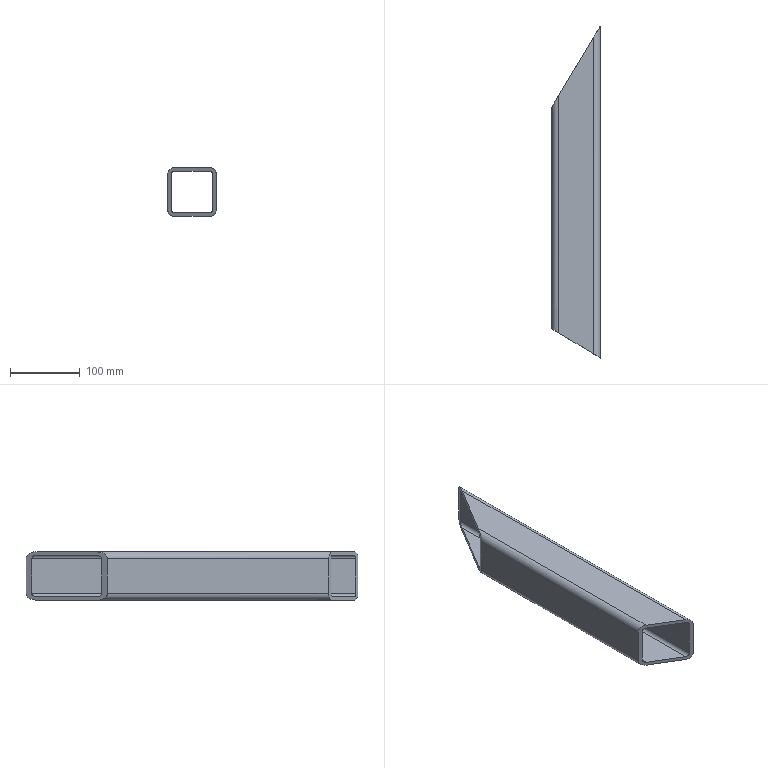Part | SolidWorks | features ICE 1, WeldMemberFeat 1, WeldmentFeature 1 | 1 solid | 18 faces | box 70 x 476 x 70 mm | volume 490129 mm3 | plane 10 | cylinder 8 | commonest cylinder face diameters 10 x4 20 x4
STEP:
#1=CARTESIAN_POINT('',(35.,0.,25.));
#2=VERTEX_POINT('',#1);
#3=CARTESIAN_POINT('',(35.,0.,-25.));
#4=VERTEX_POINT('',#3);
#5=CARTESIAN_POINT('',(35.,0.,-25.));
#6=DIRECTION('',(0.,0.,-1.));
#7=VECTOR('',#6,1000.);
#8=LINE('',#5,#7);
#9=EDGE_CURVE('',#2,#4,#8,.T.);
#10=ORIENTED_EDGE('',*,*,#9,.T.);
#11=CARTESIAN_POINT('',(35.,476.,-25.));
#12=VERTEX_POINT('',#11);
#13=CARTESIAN_POINT('',(35.,476.,-25.));
#14=DIRECTION('',(0.,-1.,0.));
#15=VECTOR('',#14,1000.);
#16=LINE('',#13,#15);
#17=EDGE_CURVE('',#12,#4,#16,.T.);
#18=ORIENTED_EDGE('',*,*,#17,.F.);
#19=CARTESIAN_POINT('',(35.,476.,25.));
#20=VERTEX_POINT('',#19);
#21=CARTESIAN_POINT('',(35.,476.,-25.));
#22=DIRECTION('',(0.,0.,-1.));
#23=VECTOR('',#22,1000.);
#24=LINE('',#21,#23);
#25=EDGE_CURVE('',#20,#12,#24,.T.);
#26=ORIENTED_EDGE('',*,*,#25,.F.);
#27=CARTESIAN_POINT('',(35.,476.,25.));
#28=DIRECTION('',(0.,-1.,0.));
#29=VECTOR('',#28,1000.);
#30=LINE('',#27,#29);
#31=EDGE_CURVE('',#20,#2,#30,.T.);
#32=ORIENTED_EDGE('',*,*,#31,.T.);
#33=EDGE_LOOP('',(#10,#18,#26,#32));
#34=FACE_OUTER_BOUND('',#33,.T.);
#35=CARTESIAN_POINT('',(35.,476.,-25.));
#36=DIRECTION('',(-1.,0.,0.));
#37=DIRECTION('',(0.,0.,1.));
#38=AXIS2_PLACEMENT_3D('',#35,#36,#37);
#39=PLANE('',#38);
#40=ADVANCED_FACE('',(#34),#39,.F.);
#41=CARTESIAN_POINT('',(-35.,359.333,25.));
#42=VERTEX_POINT('',#41);
#43=CARTESIAN_POINT('',(-35.,42.,25.));
#44=VERTEX_POINT('',#43);
#45=CARTESIAN_POINT('',(-35.,476.,25.));
#46=DIRECTION('',(0.,-1.,0.));
#47=VECTOR('',#46,1000.);
#48=LINE('',#45,#47);
#49=EDGE_CURVE('',#42,#44,#48,.T.);
#50=ORIENTED_EDGE('',*,*,#49,.F.);
#51=CARTESIAN_POINT('',(-35.,359.333,-25.));
#52=VERTEX_POINT('',#51);
#53=CARTESIAN_POINT('',(-35.,359.333,-35.));
#54=DIRECTION('',(0.,0.,1.));
#55=VECTOR('',#54,1000.);
#56=LINE('',#53,#55);
#57=EDGE_CURVE('',#52,#42,#56,.T.);
#58=ORIENTED_EDGE('',*,*,#57,.F.);
#59=CARTESIAN_POINT('',(-35.,42.,-25.));
#60=VERTEX_POINT('',#59);
#61=CARTESIAN_POINT('',(-35.,476.,-25.));
#62=DIRECTION('',(0.,-1.,0.));
#63=VECTOR('',#62,1000.);
#64=LINE('',#61,#63);
#65=EDGE_CURVE('',#52,#60,#64,.T.);
#66=ORIENTED_EDGE('',*,*,#65,.T.);
#67=CARTESIAN_POINT('',(-35.,42.,-35.));
#68=DIRECTION('',(0.,0.,1.));
#69=VECTOR('',#68,1000.);
#70=LINE('',#67,#69);
#71=EDGE_CURVE('',#60,#44,#70,.T.);
#72=ORIENTED_EDGE('',*,*,#71,.T.);
#73=EDGE_LOOP('',(#50,#58,#66,#72));
#74=FACE_OUTER_BOUND('',#73,.T.);
#75=CARTESIAN_POINT('',(-35.,476.,25.));
#76=DIRECTION('',(1.,0.,0.));
#77=DIRECTION('',(0.,0.,-1.));
#78=AXIS2_PLACEMENT_3D('',#75,#76,#77);
#79=PLANE('',#78);
#80=ADVANCED_FACE('',(#74),#79,.F.);
#81=ORIENTED_EDGE('',*,*,#65,.F.);
#82=CARTESIAN_POINT('',(-25.,376.,-35.));
#83=VERTEX_POINT('',#82);
#84=CARTESIAN_POINT('',(-35.,359.333,-25.));
#85=CARTESIAN_POINT('',(-35.,359.333,-30.858));
#86=CARTESIAN_POINT('',(-30.858,366.237,-35.));
#87=CARTESIAN_POINT('',(-25.,376.,-35.));
#88=(BOUNDED_CURVE()B_SPLINE_CURVE(3,(#84,#85,#86,#87),.UNSPECIFIED.,.F.,.F.)B_SPLINE_CURVE_WITH_KNOTS((4,4),(0.,1.571),.UNSPECIFIED.)CURVE()GEOMETRIC_REPRESENTATION_ITEM()RATIONAL_B_SPLINE_CURVE((1.,0.8047,0.8047,1.))REPRESENTATION_ITEM(''));
#89=EDGE_CURVE('',#52,#83,#88,.T.);
#90=ORIENTED_EDGE('',*,*,#89,.T.);
#91=CARTESIAN_POINT('',(-25.,36.,-35.));
#92=VERTEX_POINT('',#91);
#93=CARTESIAN_POINT('',(-25.,476.,-35.));
#94=DIRECTION('',(0.,-1.,0.));
#95=VECTOR('',#94,1000.);
#96=LINE('',#93,#95);
#97=EDGE_CURVE('',#83,#92,#96,.T.);
#98=ORIENTED_EDGE('',*,*,#97,.T.);
#99=CARTESIAN_POINT('',(-25.,36.,-35.));
#100=CARTESIAN_POINT('',(-30.858,39.515,-35.));
#101=CARTESIAN_POINT('',(-35.,42.,-30.858));
#102=CARTESIAN_POINT('',(-35.,42.,-25.));
#103=(BOUNDED_CURVE()B_SPLINE_CURVE(3,(#99,#100,#101,#102),.UNSPECIFIED.,.F.,.T.)B_SPLINE_CURVE_WITH_KNOTS((4,4),(1.571,3.142),.UNSPECIFIED.)CURVE()GEOMETRIC_REPRESENTATION_ITEM()RATIONAL_B_SPLINE_CURVE((1.,0.8047,0.8047,1.))REPRESENTATION_ITEM(''));
#104=EDGE_CURVE('',#92,#60,#103,.T.);
#105=ORIENTED_EDGE('',*,*,#104,.T.);
#106=EDGE_LOOP('',(#81,#90,#98,#105));
#107=FACE_OUTER_BOUND('',#106,.T.);
#108=CARTESIAN_POINT('',(-25.,476.,-25.));
#109=DIRECTION('',(0.,-1.,0.));
#110=DIRECTION('',(0.,0.,-1.));
#111=AXIS2_PLACEMENT_3D('',#108,#109,#110);
#112=CYLINDRICAL_SURFACE('',#111,10.);
#113=ADVANCED_FACE('',(#107),#112,.T.);
#114=ORIENTED_EDGE('',*,*,#97,.F.);
#115=CARTESIAN_POINT('',(25.,459.333,-35.));
#116=VERTEX_POINT('',#115);
#117=CARTESIAN_POINT('',(35.,476.,-35.));
#118=DIRECTION('',(0.5145,0.8575,0.));
#119=VECTOR('',#118,1000.);
#120=LINE('',#117,#119);
#121=EDGE_CURVE('',#83,#116,#120,.T.);
#122=ORIENTED_EDGE('',*,*,#121,.T.);
#123=CARTESIAN_POINT('',(25.,6.,-35.));
#124=VERTEX_POINT('',#123);
#125=CARTESIAN_POINT('',(25.,476.,-35.));
#126=DIRECTION('',(0.,-1.,0.));
#127=VECTOR('',#126,1000.);
#128=LINE('',#125,#127);
#129=EDGE_CURVE('',#116,#124,#128,.T.);
#130=ORIENTED_EDGE('',*,*,#129,.T.);
#131=CARTESIAN_POINT('',(-35.,42.,-35.));
#132=DIRECTION('',(-0.8575,0.5145,0.));
#133=VECTOR('',#132,1000.);
#134=LINE('',#131,#133);
#135=EDGE_CURVE('',#124,#92,#134,.T.);
#136=ORIENTED_EDGE('',*,*,#135,.T.);
#137=EDGE_LOOP('',(#114,#122,#130,#136));
#138=FACE_OUTER_BOUND('',#137,.T.);
#139=CARTESIAN_POINT('',(25.,476.,-35.));
#140=DIRECTION('',(0.,0.,1.));
#141=DIRECTION('',(1.,0.,0.));
#142=AXIS2_PLACEMENT_3D('',#139,#140,#141);
#143=PLANE('',#142);
#144=ADVANCED_FACE('',(#138),#143,.F.);
#145=ORIENTED_EDGE('',*,*,#129,.F.);
#146=CARTESIAN_POINT('',(25.,459.333,-35.));
#147=CARTESIAN_POINT('',(30.858,469.096,-35.));
#148=CARTESIAN_POINT('',(35.,476.,-30.858));
#149=CARTESIAN_POINT('',(35.,476.,-25.));
#150=(BOUNDED_CURVE()B_SPLINE_CURVE(3,(#146,#147,#148,#149),.UNSPECIFIED.,.F.,.F.)B_SPLINE_CURVE_WITH_KNOTS((4,4),(1.571,3.142),.UNSPECIFIED.)CURVE()GEOMETRIC_REPRESENTATION_ITEM()RATIONAL_B_SPLINE_CURVE((1.,0.8047,0.8047,1.))REPRESENTATION_ITEM(''));
#151=EDGE_CURVE('',#116,#12,#150,.T.);
#152=ORIENTED_EDGE('',*,*,#151,.T.);
#153=ORIENTED_EDGE('',*,*,#17,.T.);
#154=CARTESIAN_POINT('',(35.,0.,-25.));
#155=CARTESIAN_POINT('',(35.,0.,-30.858));
#156=CARTESIAN_POINT('',(30.858,2.485,-35.));
#157=CARTESIAN_POINT('',(25.,6.,-35.));
#158=(BOUNDED_CURVE()B_SPLINE_CURVE(3,(#154,#155,#156,#157),.UNSPECIFIED.,.F.,.F.)B_SPLINE_CURVE_WITH_KNOTS((4,4),(0.,1.571),.UNSPECIFIED.)CURVE()GEOMETRIC_REPRESENTATION_ITEM()RATIONAL_B_SPLINE_CURVE((1.,0.8047,0.8047,1.))REPRESENTATION_ITEM(''));
#159=EDGE_CURVE('',#4,#124,#158,.T.);
#160=ORIENTED_EDGE('',*,*,#159,.T.);
#161=EDGE_LOOP('',(#145,#152,#153,#160));
#162=FACE_OUTER_BOUND('',#161,.T.);
#163=CARTESIAN_POINT('',(25.,476.,-25.));
#164=DIRECTION('',(0.,-1.,0.));
#165=DIRECTION('',(0.,0.,-1.));
#166=AXIS2_PLACEMENT_3D('',#163,#164,#165);
#167=CYLINDRICAL_SURFACE('',#166,10.);
#168=ADVANCED_FACE('',(#162),#167,.T.);
#169=ORIENTED_EDGE('',*,*,#31,.F.);
#170=CARTESIAN_POINT('',(25.,459.333,35.));
#171=VERTEX_POINT('',#170);
#172=CARTESIAN_POINT('',(35.,476.,25.));
#173=CARTESIAN_POINT('',(35.,476.,30.858));
#174=CARTESIAN_POINT('',(30.858,469.096,35.));
#175=CARTESIAN_POINT('',(25.,459.333,35.));
#176=(BOUNDED_CURVE()B_SPLINE_CURVE(3,(#172,#173,#174,#175),.UNSPECIFIED.,.F.,.F.)B_SPLINE_CURVE_WITH_KNOTS((4,4),(3.142,4.712),.UNSPECIFIED.)CURVE()GEOMETRIC_REPRESENTATION_ITEM()RATIONAL_B_SPLINE_CURVE((1.,0.8047,0.8047,1.))REPRESENTATION_ITEM(''));
#177=EDGE_CURVE('',#20,#171,#176,.T.);
#178=ORIENTED_EDGE('',*,*,#177,.T.);
#179=CARTESIAN_POINT('',(25.,6.,35.));
#180=VERTEX_POINT('',#179);
#181=CARTESIAN_POINT('',(25.,476.,35.));
#182=DIRECTION('',(0.,-1.,0.));
#183=VECTOR('',#182,1000.);
#184=LINE('',#181,#183);
#185=EDGE_CURVE('',#171,#180,#184,.T.);
#186=ORIENTED_EDGE('',*,*,#185,.T.);
#187=CARTESIAN_POINT('',(25.,6.,35.));
#188=CARTESIAN_POINT('',(30.858,2.485,35.));
#189=CARTESIAN_POINT('',(35.,0.,30.858));
#190=CARTESIAN_POINT('',(35.,0.,25.));
#191=(BOUNDED_CURVE()B_SPLINE_CURVE(3,(#187,#188,#189,#190),.UNSPECIFIED.,.F.,.T.)B_SPLINE_CURVE_WITH_KNOTS((4,4),(4.712,6.283),.UNSPECIFIED.)CURVE()GEOMETRIC_REPRESENTATION_ITEM()RATIONAL_B_SPLINE_CURVE((1.,0.8047,0.8047,1.))REPRESENTATION_ITEM(''));
#192=EDGE_CURVE('',#180,#2,#191,.T.);
#193=ORIENTED_EDGE('',*,*,#192,.T.);
#194=EDGE_LOOP('',(#169,#178,#186,#193));
#195=FACE_OUTER_BOUND('',#194,.T.);
#196=CARTESIAN_POINT('',(25.,476.,25.));
#197=DIRECTION('',(0.,-1.,0.));
#198=DIRECTION('',(0.,0.,-1.));
#199=AXIS2_PLACEMENT_3D('',#196,#197,#198);
#200=CYLINDRICAL_SURFACE('',#199,10.);
#201=ADVANCED_FACE('',(#195),#200,.T.);
#202=ORIENTED_EDGE('',*,*,#185,.F.);
#203=CARTESIAN_POINT('',(-25.,376.,35.));
#204=VERTEX_POINT('',#203);
#205=CARTESIAN_POINT('',(19.118,449.529,35.));
#206=DIRECTION('',(-0.5145,-0.8575,0.));
#207=VECTOR('',#206,1000.);
#208=LINE('',#205,#207);
#209=EDGE_CURVE('',#171,#204,#208,.T.);
#210=ORIENTED_EDGE('',*,*,#209,.T.);
#211=CARTESIAN_POINT('',(-25.,36.,35.));
#212=VERTEX_POINT('',#211);
#213=CARTESIAN_POINT('',(-25.,476.,35.));
#214=DIRECTION('',(0.,-1.,0.));
#215=VECTOR('',#214,1000.);
#216=LINE('',#213,#215);
#217=EDGE_CURVE('',#204,#212,#216,.T.);
#218=ORIENTED_EDGE('',*,*,#217,.T.);
#219=CARTESIAN_POINT('',(-219.118,152.471,35.));
#220=DIRECTION('',(0.8575,-0.5145,0.));
#221=VECTOR('',#220,1000.);
#222=LINE('',#219,#221);
#223=EDGE_CURVE('',#212,#180,#222,.T.);
#224=ORIENTED_EDGE('',*,*,#223,.T.);
#225=EDGE_LOOP('',(#202,#210,#218,#224));
#226=FACE_OUTER_BOUND('',#225,.T.);
#227=CARTESIAN_POINT('',(-25.,476.,35.));
#228=DIRECTION('',(0.,0.,-1.));
#229=DIRECTION('',(-1.,0.,0.));
#230=AXIS2_PLACEMENT_3D('',#227,#228,#229);
#231=PLANE('',#230);
#232=ADVANCED_FACE('',(#226),#231,.F.);
#233=ORIENTED_EDGE('',*,*,#217,.F.);
#234=CARTESIAN_POINT('',(-25.,376.,35.));
#235=CARTESIAN_POINT('',(-30.858,366.237,35.));
#236=CARTESIAN_POINT('',(-35.,359.333,30.858));
#237=CARTESIAN_POINT('',(-35.,359.333,25.));
#238=(BOUNDED_CURVE()B_SPLINE_CURVE(3,(#234,#235,#236,#237),.UNSPECIFIED.,.F.,.F.)B_SPLINE_CURVE_WITH_KNOTS((4,4),(4.712,6.283),.UNSPECIFIED.)CURVE()GEOMETRIC_REPRESENTATION_ITEM()RATIONAL_B_SPLINE_CURVE((1.,0.8047,0.8047,1.))REPRESENTATION_ITEM(''));
#239=EDGE_CURVE('',#204,#42,#238,.T.);
#240=ORIENTED_EDGE('',*,*,#239,.T.);
#241=ORIENTED_EDGE('',*,*,#49,.T.);
#242=CARTESIAN_POINT('',(-35.,42.,25.));
#243=CARTESIAN_POINT('',(-35.,42.,30.858));
#244=CARTESIAN_POINT('',(-30.858,39.515,35.));
#245=CARTESIAN_POINT('',(-25.,36.,35.));
#246=(BOUNDED_CURVE()B_SPLINE_CURVE(3,(#242,#243,#244,#245),.UNSPECIFIED.,.F.,.T.)B_SPLINE_CURVE_WITH_KNOTS((4,4),(3.142,4.712),.UNSPECIFIED.)CURVE()GEOMETRIC_REPRESENTATION_ITEM()RATIONAL_B_SPLINE_CURVE((1.,0.8047,0.8047,1.))REPRESENTATION_ITEM(''));
#247=EDGE_CURVE('',#44,#212,#246,.T.);
#248=ORIENTED_EDGE('',*,*,#247,.T.);
#249=EDGE_LOOP('',(#233,#240,#241,#248));
#250=FACE_OUTER_BOUND('',#249,.T.);
#251=CARTESIAN_POINT('',(-25.,476.,25.));
#252=DIRECTION('',(0.,-1.,0.));
#253=DIRECTION('',(0.,0.,-1.));
#254=AXIS2_PLACEMENT_3D('',#251,#252,#253);
#255=CYLINDRICAL_SURFACE('',#254,10.);
#256=ADVANCED_FACE('',(#250),#255,.T.);
#257=CARTESIAN_POINT('',(25.,6.,30.));
#258=VERTEX_POINT('',#257);
#259=CARTESIAN_POINT('',(30.,3.,25.));
#260=VERTEX_POINT('',#259);
#261=CARTESIAN_POINT('',(25.,6.,30.));
#262=CARTESIAN_POINT('',(27.929,4.243,30.));
#263=CARTESIAN_POINT('',(30.,3.,27.929));
#264=CARTESIAN_POINT('',(30.,3.,25.));
#265=(BOUNDED_CURVE()B_SPLINE_CURVE(3,(#261,#262,#263,#264),.UNSPECIFIED.,.F.,.F.)B_SPLINE_CURVE_WITH_KNOTS((4,4),(4.712,6.283),.UNSPECIFIED.)CURVE()GEOMETRIC_REPRESENTATION_ITEM()RATIONAL_B_SPLINE_CURVE((1.,0.8047,0.8047,1.))REPRESENTATION_ITEM(''));
#266=EDGE_CURVE('',#258,#260,#265,.T.);
#267=ORIENTED_EDGE('',*,*,#266,.T.);
#268=CARTESIAN_POINT('',(30.,3.,-25.));
#269=VERTEX_POINT('',#268);
#270=CARTESIAN_POINT('',(30.,3.,-25.));
#271=DIRECTION('',(0.,0.,-1.));
#272=VECTOR('',#271,1000.);
#273=LINE('',#270,#272);
#274=EDGE_CURVE('',#260,#269,#273,.T.);
#275=ORIENTED_EDGE('',*,*,#274,.T.);
#276=CARTESIAN_POINT('',(25.,6.,-30.));
#277=VERTEX_POINT('',#276);
#278=CARTESIAN_POINT('',(30.,3.,-25.));
#279=CARTESIAN_POINT('',(30.,3.,-27.929));
#280=CARTESIAN_POINT('',(27.929,4.243,-30.));
#281=CARTESIAN_POINT('',(25.,6.,-30.));
#282=(BOUNDED_CURVE()B_SPLINE_CURVE(3,(#278,#279,#280,#281),.UNSPECIFIED.,.F.,.F.)B_SPLINE_CURVE_WITH_KNOTS((4,4),(0.,1.571),.UNSPECIFIED.)CURVE()GEOMETRIC_REPRESENTATION_ITEM()RATIONAL_B_SPLINE_CURVE((1.,0.8047,0.8047,1.))REPRESENTATION_ITEM(''));
#283=EDGE_CURVE('',#269,#277,#282,.T.);
#284=ORIENTED_EDGE('',*,*,#283,.T.);
#285=CARTESIAN_POINT('',(-25.,36.,-30.));
#286=VERTEX_POINT('',#285);
#287=CARTESIAN_POINT('',(-182.353,130.412,-30.));
#288=DIRECTION('',(-0.8575,0.5145,0.));
#289=VECTOR('',#288,1000.);
#290=LINE('',#287,#289);
#291=EDGE_CURVE('',#277,#286,#290,.T.);
#292=ORIENTED_EDGE('',*,*,#291,.T.);
#293=CARTESIAN_POINT('',(-30.,39.,-25.));
#294=VERTEX_POINT('',#293);
#295=CARTESIAN_POINT('',(-25.,36.,-30.));
#296=CARTESIAN_POINT('',(-27.929,37.757,-30.));
#297=CARTESIAN_POINT('',(-30.,39.,-27.929));
#298=CARTESIAN_POINT('',(-30.,39.,-25.));
#299=(BOUNDED_CURVE()B_SPLINE_CURVE(3,(#295,#296,#297,#298),.UNSPECIFIED.,.F.,.F.)B_SPLINE_CURVE_WITH_KNOTS((4,4),(1.571,3.142),.UNSPECIFIED.)CURVE()GEOMETRIC_REPRESENTATION_ITEM()RATIONAL_B_SPLINE_CURVE((1.,0.8047,0.8047,1.))REPRESENTATION_ITEM(''));
#300=EDGE_CURVE('',#286,#294,#299,.T.);
#301=ORIENTED_EDGE('',*,*,#300,.T.);
#302=CARTESIAN_POINT('',(-30.,39.,25.));
#303=VERTEX_POINT('',#302);
#304=CARTESIAN_POINT('',(-30.,39.,25.));
#305=DIRECTION('',(0.,0.,1.));
#306=VECTOR('',#305,1000.);
#307=LINE('',#304,#306);
#308=EDGE_CURVE('',#294,#303,#307,.T.);
#309=ORIENTED_EDGE('',*,*,#308,.T.);
#310=CARTESIAN_POINT('',(-25.,36.,30.));
#311=VERTEX_POINT('',#310);
#312=CARTESIAN_POINT('',(-30.,39.,25.));
#313=CARTESIAN_POINT('',(-30.,39.,27.929));
#314=CARTESIAN_POINT('',(-27.929,37.757,30.));
#315=CARTESIAN_POINT('',(-25.,36.,30.));
#316=(BOUNDED_CURVE()B_SPLINE_CURVE(3,(#312,#313,#314,#315),.UNSPECIFIED.,.F.,.F.)B_SPLINE_CURVE_WITH_KNOTS((4,4),(3.142,4.712),.UNSPECIFIED.)CURVE()GEOMETRIC_REPRESENTATION_ITEM()RATIONAL_B_SPLINE_CURVE((1.,0.8047,0.8047,1.))REPRESENTATION_ITEM(''));
#317=EDGE_CURVE('',#303,#311,#316,.T.);
#318=ORIENTED_EDGE('',*,*,#317,.T.);
#319=CARTESIAN_POINT('',(-219.118,152.471,30.));
#320=DIRECTION('',(0.8575,-0.5145,0.));
#321=VECTOR('',#320,1000.);
#322=LINE('',#319,#321);
#323=EDGE_CURVE('',#311,#258,#322,.T.);
#324=ORIENTED_EDGE('',*,*,#323,.T.);
#325=EDGE_LOOP('',(#267,#275,#284,#292,#301,#309,#318,#324));
#326=FACE_BOUND('',#325,.T.);
#327=ORIENTED_EDGE('',*,*,#71,.F.);
#328=ORIENTED_EDGE('',*,*,#104,.F.);
#329=ORIENTED_EDGE('',*,*,#135,.F.);
#330=ORIENTED_EDGE('',*,*,#159,.F.);
#331=ORIENTED_EDGE('',*,*,#9,.F.);
#332=ORIENTED_EDGE('',*,*,#192,.F.);
#333=ORIENTED_EDGE('',*,*,#223,.F.);
#334=ORIENTED_EDGE('',*,*,#247,.F.);
#335=EDGE_LOOP('',(#327,#328,#329,#330,#331,#332,#333,#334));
#336=FACE_OUTER_BOUND('',#335,.T.);
#337=CARTESIAN_POINT('',(-35.,42.,-35.));
#338=DIRECTION('',(0.5145,0.8575,0.));
#339=DIRECTION('',(-0.8575,0.5145,0.));
#340=AXIS2_PLACEMENT_3D('',#337,#338,#339);
#341=PLANE('',#340);
#342=ADVANCED_FACE('',(#326,#336),#341,.F.);
#343=CARTESIAN_POINT('',(30.,467.667,25.));
#344=VERTEX_POINT('',#343);
#345=CARTESIAN_POINT('',(25.,459.333,30.));
#346=VERTEX_POINT('',#345);
#347=CARTESIAN_POINT('',(30.,467.667,25.));
#348=CARTESIAN_POINT('',(30.,467.667,27.929));
#349=CARTESIAN_POINT('',(27.929,464.215,30.));
#350=CARTESIAN_POINT('',(25.,459.333,30.));
#351=(BOUNDED_CURVE()B_SPLINE_CURVE(3,(#347,#348,#349,#350),.UNSPECIFIED.,.F.,.F.)B_SPLINE_CURVE_WITH_KNOTS((4,4),(3.142,4.712),.UNSPECIFIED.)CURVE()GEOMETRIC_REPRESENTATION_ITEM()RATIONAL_B_SPLINE_CURVE((1.,0.8047,0.8047,1.))REPRESENTATION_ITEM(''));
#352=EDGE_CURVE('',#344,#346,#351,.T.);
#353=ORIENTED_EDGE('',*,*,#352,.T.);
#354=CARTESIAN_POINT('',(-25.,376.,30.));
#355=VERTEX_POINT('',#354);
#356=CARTESIAN_POINT('',(19.118,449.529,30.));
#357=DIRECTION('',(-0.5145,-0.8575,0.));
#358=VECTOR('',#357,1000.);
#359=LINE('',#356,#358);
#360=EDGE_CURVE('',#346,#355,#359,.T.);
#361=ORIENTED_EDGE('',*,*,#360,.T.);
#362=CARTESIAN_POINT('',(-30.,367.667,25.));
#363=VERTEX_POINT('',#362);
#364=CARTESIAN_POINT('',(-25.,376.,30.));
#365=CARTESIAN_POINT('',(-27.929,371.118,30.));
#366=CARTESIAN_POINT('',(-30.,367.667,27.929));
#367=CARTESIAN_POINT('',(-30.,367.667,25.));
#368=(BOUNDED_CURVE()B_SPLINE_CURVE(3,(#364,#365,#366,#367),.UNSPECIFIED.,.F.,.T.)B_SPLINE_CURVE_WITH_KNOTS((4,4),(4.712,6.283),.UNSPECIFIED.)CURVE()GEOMETRIC_REPRESENTATION_ITEM()RATIONAL_B_SPLINE_CURVE((1.,0.8047,0.8047,1.))REPRESENTATION_ITEM(''));
#369=EDGE_CURVE('',#355,#363,#368,.T.);
#370=ORIENTED_EDGE('',*,*,#369,.T.);
#371=CARTESIAN_POINT('',(-30.,367.667,-25.));
#372=VERTEX_POINT('',#371);
#373=CARTESIAN_POINT('',(-30.,367.667,25.));
#374=DIRECTION('',(0.,0.,-1.));
#375=VECTOR('',#374,1000.);
#376=LINE('',#373,#375);
#377=EDGE_CURVE('',#363,#372,#376,.T.);
#378=ORIENTED_EDGE('',*,*,#377,.T.);
#379=CARTESIAN_POINT('',(-25.,376.,-30.));
#380=VERTEX_POINT('',#379);
#381=CARTESIAN_POINT('',(-30.,367.667,-25.));
#382=CARTESIAN_POINT('',(-30.,367.667,-27.929));
#383=CARTESIAN_POINT('',(-27.929,371.118,-30.));
#384=CARTESIAN_POINT('',(-25.,376.,-30.));
#385=(BOUNDED_CURVE()B_SPLINE_CURVE(3,(#381,#382,#383,#384),.UNSPECIFIED.,.F.,.F.)B_SPLINE_CURVE_WITH_KNOTS((4,4),(0.,1.571),.UNSPECIFIED.)CURVE()GEOMETRIC_REPRESENTATION_ITEM()RATIONAL_B_SPLINE_CURVE((1.,0.8047,0.8047,1.))REPRESENTATION_ITEM(''));
#386=EDGE_CURVE('',#372,#380,#385,.T.);
#387=ORIENTED_EDGE('',*,*,#386,.T.);
#388=CARTESIAN_POINT('',(25.,459.333,-30.));
#389=VERTEX_POINT('',#388);
#390=CARTESIAN_POINT('',(32.353,471.588,-30.));
#391=DIRECTION('',(0.5145,0.8575,0.));
#392=VECTOR('',#391,1000.);
#393=LINE('',#390,#392);
#394=EDGE_CURVE('',#380,#389,#393,.T.);
#395=ORIENTED_EDGE('',*,*,#394,.T.);
#396=CARTESIAN_POINT('',(30.,467.667,-25.));
#397=VERTEX_POINT('',#396);
#398=CARTESIAN_POINT('',(25.,459.333,-30.));
#399=CARTESIAN_POINT('',(27.929,464.215,-30.));
#400=CARTESIAN_POINT('',(30.,467.667,-27.929));
#401=CARTESIAN_POINT('',(30.,467.667,-25.));
#402=(BOUNDED_CURVE()B_SPLINE_CURVE(3,(#398,#399,#400,#401),.UNSPECIFIED.,.F.,.F.)B_SPLINE_CURVE_WITH_KNOTS((4,4),(1.571,3.142),.UNSPECIFIED.)CURVE()GEOMETRIC_REPRESENTATION_ITEM()RATIONAL_B_SPLINE_CURVE((1.,0.8047,0.8047,1.))REPRESENTATION_ITEM(''));
#403=EDGE_CURVE('',#389,#397,#402,.T.);
#404=ORIENTED_EDGE('',*,*,#403,.T.);
#405=CARTESIAN_POINT('',(30.,467.667,-25.));
#406=DIRECTION('',(0.,0.,1.));
#407=VECTOR('',#406,1000.);
#408=LINE('',#405,#407);
#409=EDGE_CURVE('',#397,#344,#408,.T.);
#410=ORIENTED_EDGE('',*,*,#409,.T.);
#411=EDGE_LOOP('',(#353,#361,#370,#378,#387,#395,#404,#410));
#412=FACE_BOUND('',#411,.T.);
#413=ORIENTED_EDGE('',*,*,#209,.F.);
#414=ORIENTED_EDGE('',*,*,#177,.F.);
#415=ORIENTED_EDGE('',*,*,#25,.T.);
#416=ORIENTED_EDGE('',*,*,#151,.F.);
#417=ORIENTED_EDGE('',*,*,#121,.F.);
#418=ORIENTED_EDGE('',*,*,#89,.F.);
#419=ORIENTED_EDGE('',*,*,#57,.T.);
#420=ORIENTED_EDGE('',*,*,#239,.F.);
#421=EDGE_LOOP('',(#413,#414,#415,#416,#417,#418,#419,#420));
#422=FACE_OUTER_BOUND('',#421,.T.);
#423=CARTESIAN_POINT('',(35.,476.,-35.));
#424=DIRECTION('',(0.8575,-0.5145,0.));
#425=DIRECTION('',(0.5145,0.8575,0.));
#426=AXIS2_PLACEMENT_3D('',#423,#424,#425);
#427=PLANE('',#426);
#428=ADVANCED_FACE('',(#412,#422),#427,.F.);
#429=ORIENTED_EDGE('',*,*,#352,.F.);
#430=CARTESIAN_POINT('',(30.,476.,25.));
#431=DIRECTION('',(0.,-1.,0.));
#432=VECTOR('',#431,1000.);
#433=LINE('',#430,#432);
#434=EDGE_CURVE('',#344,#260,#433,.T.);
#435=ORIENTED_EDGE('',*,*,#434,.T.);
#436=ORIENTED_EDGE('',*,*,#266,.F.);
#437=CARTESIAN_POINT('',(25.,476.,30.));
#438=DIRECTION('',(0.,-1.,0.));
#439=VECTOR('',#438,1000.);
#440=LINE('',#437,#439);
#441=EDGE_CURVE('',#346,#258,#440,.T.);
#442=ORIENTED_EDGE('',*,*,#441,.F.);
#443=EDGE_LOOP('',(#429,#435,#436,#442));
#444=FACE_OUTER_BOUND('',#443,.T.);
#445=CARTESIAN_POINT('',(25.,476.,25.));
#446=DIRECTION('',(0.,-1.,0.));
#447=DIRECTION('',(0.,0.,-1.));
#448=AXIS2_PLACEMENT_3D('',#445,#446,#447);
#449=CYLINDRICAL_SURFACE('',#448,5.);
#450=ADVANCED_FACE('',(#444),#449,.F.);
#451=ORIENTED_EDGE('',*,*,#360,.F.);
#452=ORIENTED_EDGE('',*,*,#441,.T.);
#453=ORIENTED_EDGE('',*,*,#323,.F.);
#454=CARTESIAN_POINT('',(-25.,476.,30.));
#455=DIRECTION('',(0.,-1.,0.));
#456=VECTOR('',#455,1000.);
#457=LINE('',#454,#456);
#458=EDGE_CURVE('',#355,#311,#457,.T.);
#459=ORIENTED_EDGE('',*,*,#458,.F.);
#460=EDGE_LOOP('',(#451,#452,#453,#459));
#461=FACE_OUTER_BOUND('',#460,.T.);
#462=CARTESIAN_POINT('',(-25.,476.,30.));
#463=DIRECTION('',(0.,0.,-1.));
#464=DIRECTION('',(-1.,0.,0.));
#465=AXIS2_PLACEMENT_3D('',#462,#463,#464);
#466=PLANE('',#465);
#467=ADVANCED_FACE('',(#461),#466,.T.);
#468=ORIENTED_EDGE('',*,*,#369,.F.);
#469=ORIENTED_EDGE('',*,*,#458,.T.);
#470=ORIENTED_EDGE('',*,*,#317,.F.);
#471=CARTESIAN_POINT('',(-30.,476.,25.));
#472=DIRECTION('',(0.,-1.,0.));
#473=VECTOR('',#472,1000.);
#474=LINE('',#471,#473);
#475=EDGE_CURVE('',#363,#303,#474,.T.);
#476=ORIENTED_EDGE('',*,*,#475,.F.);
#477=EDGE_LOOP('',(#468,#469,#470,#476));
#478=FACE_OUTER_BOUND('',#477,.T.);
#479=CARTESIAN_POINT('',(-25.,476.,25.));
#480=DIRECTION('',(0.,-1.,0.));
#481=DIRECTION('',(0.,0.,-1.));
#482=AXIS2_PLACEMENT_3D('',#479,#480,#481);
#483=CYLINDRICAL_SURFACE('',#482,5.);
#484=ADVANCED_FACE('',(#478),#483,.F.);
#485=ORIENTED_EDGE('',*,*,#377,.F.);
#486=ORIENTED_EDGE('',*,*,#475,.T.);
#487=ORIENTED_EDGE('',*,*,#308,.F.);
#488=CARTESIAN_POINT('',(-30.,476.,-25.));
#489=DIRECTION('',(0.,-1.,0.));
#490=VECTOR('',#489,1000.);
#491=LINE('',#488,#490);
#492=EDGE_CURVE('',#372,#294,#491,.T.);
#493=ORIENTED_EDGE('',*,*,#492,.F.);
#494=EDGE_LOOP('',(#485,#486,#487,#493));
#495=FACE_OUTER_BOUND('',#494,.T.);
#496=CARTESIAN_POINT('',(-30.,476.,25.));
#497=DIRECTION('',(1.,0.,0.));
#498=DIRECTION('',(0.,0.,-1.));
#499=AXIS2_PLACEMENT_3D('',#496,#497,#498);
#500=PLANE('',#499);
#501=ADVANCED_FACE('',(#495),#500,.T.);
#502=ORIENTED_EDGE('',*,*,#386,.F.);
#503=ORIENTED_EDGE('',*,*,#492,.T.);
#504=ORIENTED_EDGE('',*,*,#300,.F.);
#505=CARTESIAN_POINT('',(-25.,476.,-30.));
#506=DIRECTION('',(0.,-1.,0.));
#507=VECTOR('',#506,1000.);
#508=LINE('',#505,#507);
#509=EDGE_CURVE('',#380,#286,#508,.T.);
#510=ORIENTED_EDGE('',*,*,#509,.F.);
#511=EDGE_LOOP('',(#502,#503,#504,#510));
#512=FACE_OUTER_BOUND('',#511,.T.);
#513=CARTESIAN_POINT('',(-25.,476.,-25.));
#514=DIRECTION('',(0.,-1.,0.));
#515=DIRECTION('',(0.,0.,-1.));
#516=AXIS2_PLACEMENT_3D('',#513,#514,#515);
#517=CYLINDRICAL_SURFACE('',#516,5.);
#518=ADVANCED_FACE('',(#512),#517,.F.);
#519=ORIENTED_EDGE('',*,*,#394,.F.);
#520=ORIENTED_EDGE('',*,*,#509,.T.);
#521=ORIENTED_EDGE('',*,*,#291,.F.);
#522=CARTESIAN_POINT('',(25.,476.,-30.));
#523=DIRECTION('',(0.,-1.,0.));
#524=VECTOR('',#523,1000.);
#525=LINE('',#522,#524);
#526=EDGE_CURVE('',#389,#277,#525,.T.);
#527=ORIENTED_EDGE('',*,*,#526,.F.);
#528=EDGE_LOOP('',(#519,#520,#521,#527));
#529=FACE_OUTER_BOUND('',#528,.T.);
#530=CARTESIAN_POINT('',(25.,476.,-30.));
#531=DIRECTION('',(0.,0.,1.));
#532=DIRECTION('',(1.,0.,0.));
#533=AXIS2_PLACEMENT_3D('',#530,#531,#532);
#534=PLANE('',#533);
#535=ADVANCED_FACE('',(#529),#534,.T.);
#536=ORIENTED_EDGE('',*,*,#403,.F.);
#537=ORIENTED_EDGE('',*,*,#526,.T.);
#538=ORIENTED_EDGE('',*,*,#283,.F.);
#539=CARTESIAN_POINT('',(30.,476.,-25.));
#540=DIRECTION('',(0.,-1.,0.));
#541=VECTOR('',#540,1000.);
#542=LINE('',#539,#541);
#543=EDGE_CURVE('',#397,#269,#542,.T.);
#544=ORIENTED_EDGE('',*,*,#543,.F.);
#545=EDGE_LOOP('',(#536,#537,#538,#544));
#546=FACE_OUTER_BOUND('',#545,.T.);
#547=CARTESIAN_POINT('',(25.,476.,-25.));
#548=DIRECTION('',(0.,-1.,0.));
#549=DIRECTION('',(0.,0.,-1.));
#550=AXIS2_PLACEMENT_3D('',#547,#548,#549);
#551=CYLINDRICAL_SURFACE('',#550,5.);
#552=ADVANCED_FACE('',(#546),#551,.F.);
#553=ORIENTED_EDGE('',*,*,#409,.F.);
#554=ORIENTED_EDGE('',*,*,#543,.T.);
#555=ORIENTED_EDGE('',*,*,#274,.F.);
#556=ORIENTED_EDGE('',*,*,#434,.F.);
#557=EDGE_LOOP('',(#553,#554,#555,#556));
#558=FACE_OUTER_BOUND('',#557,.T.);
#559=CARTESIAN_POINT('',(30.,476.,-25.));
#560=DIRECTION('',(-1.,0.,0.));
#561=DIRECTION('',(0.,0.,1.));
#562=AXIS2_PLACEMENT_3D('',#559,#560,#561);
#563=PLANE('',#562);
#564=ADVANCED_FACE('',(#558),#563,.T.);
#565=CLOSED_SHELL('',(#40,#80,#113,#144,#168,#201,#232,#256,#342,#428,#450,#467,#484,#501,#518,#535,#552,#564));
#566=MANIFOLD_SOLID_BREP('',#565);
#567=CARTESIAN_POINT('',(0.,0.,0.));
#568=DIRECTION('',(0.,0.,1.));
#569=DIRECTION('',(1.,0.,0.));
#570=AXIS2_PLACEMENT_3D('',#567,#568,#569);
#571=(LENGTH_UNIT()NAMED_UNIT(*)SI_UNIT(.MILLI.,.METRE.));
#572=UNCERTAINTY_MEASURE_WITH_UNIT(LENGTH_MEASURE(0.00001),#571,'','');
#573=(NAMED_UNIT(*)PLANE_ANGLE_UNIT()SI_UNIT($,.RADIAN.));
#574=(NAMED_UNIT(*)SI_UNIT($,.STERADIAN.)SOLID_ANGLE_UNIT());
#575=(GEOMETRIC_REPRESENTATION_CONTEXT(3)GLOBAL_UNCERTAINTY_ASSIGNED_CONTEXT((#572))GLOBAL_UNIT_ASSIGNED_CONTEXT((#571,#573,#574))REPRESENTATION_CONTEXT('',''));
#576=ADVANCED_BREP_SHAPE_REPRESENTATION('',(#566,#570),#575);